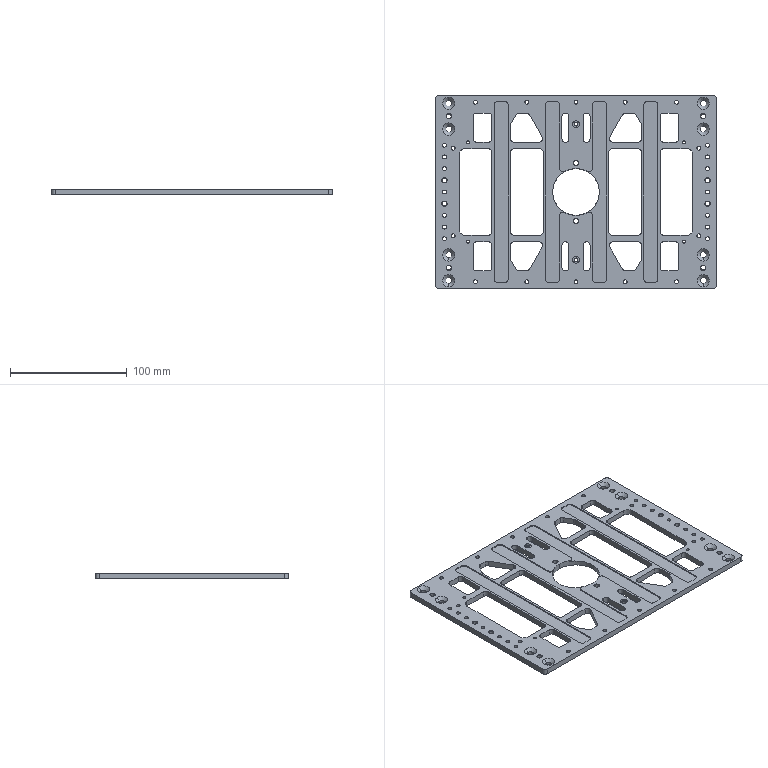NC program | NX | posted with a generic post | part box 240 x 165 x 5 mm
Lines 9636 to 10654 of 12487:
(PLANAR_MILL_COPY_COPY_COPY , TOOL : D6A45)
N19186 T01 M6
N19188 G54
N19190 G17 G0 G90 X-55.05 Y0.866 S9500 M3
N19192 G43 Z30. H1
N19194 Z0.95
N19196 G94 G1 Z-0.55 F1250.
N19198 G3 X-55.55 Y0. R1.
N19200 G1 Y-34.
N19202 G3 X-53. Y-36.55 R2.55
N19204 G1 X-31.
N19206 G3 X-28.45 Y-34. R2.55
N19208 G1 Y34.
N19210 G3 X-31. Y36.55 R2.55
N19212 G1 X-53.
N19214 G3 X-55.55 Y34. R2.55
N19216 G1 Y0.
N19218 G3 X-55.05 Y-0.866 R1.
N19220 G1 Z0.95
N19222 G0 Z30.
N19224 X-69.05 Y0.866
N19226 Z0.95
N19228 G1 Z-0.55
N19230 G3 X-69.55 Y0. R1.
N19232 G1 Y-74.5
N19234 G3 X-67. Y-77.05 R2.55
N19236 G1 X-61.
N19238 G3 X-58.45 Y-74.5 R2.55
N19240 G1 Y74.5
N19242 G3 X-61. Y77.05 R2.55
N19244 G1 X-67.
N19246 G3 X-69.55 Y74.5 R2.55
N19248 G1 Y0.
N19250 G3 X-69.05 Y-0.866 R1.
N19252 G1 Z0.95
N19254 G0 Z30.
N19256 X-99.05 Y0.866
N19258 Z0.95
N19260 G1 Z-0.55
N19262 G3 X-99.55 Y0. R1.
N19264 G1 Y-32.
N19266 G3 X-95. Y-36.55 R4.55
N19268 G1 X-75.
N19270 G3 X-72.45 Y-34. R2.55
N19272 G1 Y34.
N19274 G3 X-75. Y36.55 R2.55
N19276 G1 X-95.
N19278 G3 X-99.55 Y32. R4.55
N19280 G1 Y0.
N19282 G3 X-99.05 Y-0.866 R1.
N19284 G1 Z0.95
N19286 G0 Z30.
N19288 X-93.052 Y42.933
N19290 Z0.95
N19292 G1 Z-0.55
N19294 G3 X-93.302 Y42.5 R0.5
N19296 X-92.502 Y41.7 R0.8
N19298 X-93.302 Y42.5 R-0.8
N19300 X-93.052 Y42.067 R0.5
N19302 G1 Z0.95
N19304 G0 Z30.
N19306 X-87.05 Y55.866
N19308 Z0.95
N19310 G1 Z-0.55
N19312 G3 X-87.55 Y55. R1.
N19314 G1 Y45.5
N19316 G3 X-85. Y42.95 R2.55
N19318 G1 X-75.
N19320 G3 X-72.45 Y45.5 R2.55
N19322 G1 Y64.5
N19324 G3 X-75. Y67.05 R2.55
N19326 G1 X-85.
N19328 G3 X-87.55 Y64.5 R2.55
N19330 G1 Y55.
N19332 G3 X-87.05 Y54.134 R1.
N19334 G1 Z0.95
N19336 G0 Z30.
N19338 X-85.134 Y77.5
N19340 Z0.95
N19342 G1 Z-0.55
N19344 G3 X-86. Y78. R1.
N19346 X-87.2 Y76.8 R1.2
N19348 X-86. Y78. R-1.2
N19350 X-86.866 Y77.5 R1.
N19352 G1 Z0.95
N19354 G0 Z30.
N19356 X-107.884 Y77.45
N19358 Z0.95
N19360 G1 Z-0.55
N19362 G3 X-108.75 Y77.95 R1.
N19364 X-110.95 Y75.75 R2.2
N19366 X-108.75 Y77.95 R-2.2
N19368 X-109.616 Y77.45 R1.
N19370 G1 Z0.95
N19372 G0 Z30.
N19374 X-109.8 Y65.616
N19376 Z0.95
N19378 G1 Z-0.55
N19380 G3 X-110.3 Y64.75 R1.
N19382 X-108.75 Y63.2 R1.55
N19384 X-110.3 Y64.75 R-1.55
N19386 X-109.8 Y63.884 R1.
N19388 G1 Z0.95
N19390 G0 Z30.
N19392 X-110.45 Y54.616
N19394 Z0.95
N19396 G1 Z-0.55
N19398 G3 X-110.95 Y53.75 R1.
N19400 X-108.75 Y51.55 R2.2
N19402 X-110.95 Y53.75 R-2.2
N19404 X-110.45 Y52.884 R1.
N19406 G1 Z0.95
N19408 G0 Z30.
N19410 X-113.2 Y40.866
N19412 Z0.95
N19414 G1 Z-0.55
N19416 G3 X-113.7 Y40. R1.
N19418 X-112.5 Y38.8 R1.2
N19420 X-113.7 Y40. R-1.2
N19422 X-113.2 Y39.134 R1.
N19424 G1 Z0.95
N19426 G0 Z30.
N19428 X-105.7 Y38.366
N19430 Z0.95
N19432 G1 Z-0.55
N19434 G3 X-106.2 Y37.5 R1.
N19436 X-105. Y36.3 R1.2
N19438 X-106.2 Y37.5 R-1.2
N19440 X-105.7 Y36.634 R1.
N19442 G1 Z0.95
N19444 G0 Z30.
N19446 X-113.2 Y30.866
N19448 Z0.95
N19450 G1 Z-0.55
N19452 G3 X-113.7 Y30. R1.
N19454 X-112.5 Y28.8 R1.2
N19456 X-113.7 Y30. R-1.2
N19458 X-113.2 Y29.134 R1.
N19460 G1 Z0.95
N19462 G0 Z30.
N19464 Y20.866
N19466 Z0.95
N19468 G1 Z-0.55
N19470 G3 X-113.7 Y20. R1.
N19472 X-112.5 Y18.8 R1.2
N19474 X-113.7 Y20. R-1.2
N19476 X-113.2 Y19.134 R1.
N19478 G1 Z0.95
N19480 G0 Z30.
N19482 X-113.55 Y10.866
N19484 Z0.95
N19486 G1 Z-0.55
N19488 G3 X-114.05 Y10. R1.
N19490 X-112.5 Y8.45 R1.55
N19492 X-114.05 Y10. R-1.55
N19494 X-113.55 Y9.134 R1.
N19496 G1 Z0.95
N19498 G0 Z30.
N19500 X-113.2 Y0.866
N19502 Z0.95
N19504 G1 Z-0.55
N19506 G3 X-113.7 Y0. R1.
N19508 X-112.5 Y-1.2 R1.2
N19510 X-113.7 Y0. R-1.2
N19512 X-113.2 Y-0.866 R1.
N19514 G1 Z0.95
N19516 G0 Z30.
N19518 X-113.55 Y-9.134
N19520 Z0.95
N19522 G1 Z-0.55
N19524 G3 X-114.05 Y-10. R1.
N19526 X-112.5 Y-11.55 R1.55
N19528 X-114.05 Y-10. R-1.55
N19530 X-113.55 Y-10.866 R1.
N19532 G1 Z0.95
N19534 G0 Z30.
N19536 X-113.2 Y-19.134
N19538 Z0.95
N19540 G1 Z-0.55
N19542 G3 X-113.7 Y-20. R1.
N19544 X-112.5 Y-21.2 R1.2
N19546 X-113.7 Y-20. R-1.2
N19548 X-113.2 Y-20.866 R1.
N19550 G1 Z0.95
N19552 G0 Z30.
N19554 Y-29.134
N19556 Z0.95
N19558 G1 Z-0.55
N19560 G3 X-113.7 Y-30. R1.
N19562 X-112.5 Y-31.2 R1.2
N19564 X-113.7 Y-30. R-1.2
N19566 X-113.2 Y-30.866 R1.
N19568 G1 Z0.95
N19570 G0 Z30.
N19572 Y-39.134
N19574 Z0.95
N19576 G1 Z-0.55
N19578 G3 X-113.7 Y-40. R1.
N19580 X-112.5 Y-41.2 R1.2
N19582 X-113.7 Y-40. R-1.2
N19584 X-113.2 Y-40.866 R1.
N19586 G1 Z0.95
N19588 G0 Z30.
N19590 X-105.7 Y-36.634
N19592 Z0.95
N19594 G1 Z-0.55
N19596 G3 X-106.2 Y-37.5 R1.
N19598 X-105. Y-38.7 R1.2
N19600 X-106.2 Y-37.5 R-1.2
N19602 X-105.7 Y-38.366 R1.
N19604 G1 Z0.95
N19606 G0 Z30.
N19608 X-93.052 Y-42.069
N19610 Z0.95
N19612 G1 Z-0.55
N19614 G3 X-93.302 Y-42.502 R0.5
N19616 X-92.502 Y-43.302 R0.8
N19618 X-93.302 Y-42.502 R-0.8
N19620 X-93.052 Y-42.935 R0.5
N19622 G1 Z0.95
N19624 G0 Z30.
N19626 X-110.45 Y-52.884
N19628 Z0.95
N19630 G1 Z-0.55
N19632 G3 X-110.95 Y-53.75 R1.
N19634 X-108.75 Y-55.95 R2.2
N19636 X-110.95 Y-53.75 R-2.2
N19638 X-110.45 Y-54.616 R1.
N19640 G1 Z0.95
N19642 G0 Z30.
N19644 X-109.8 Y-63.884
N19646 Z0.95
N19648 G1 Z-0.55
N19650 G3 X-110.3 Y-64.75 R1.
N19652 X-108.75 Y-66.3 R1.55
N19654 X-110.3 Y-64.75 R-1.55
N19656 X-109.8 Y-65.616 R1.
N19658 G1 Z0.95
N19660 G0 Z30.
N19662 X-109.616 Y-77.45
N19664 Z0.95
N19666 G1 Z-0.55
N19668 G3 X-108.75 Y-77.95 R1.
N19670 X-106.55 Y-75.75 R2.2
N19672 X-108.75 Y-77.95 R-2.2
N19674 X-107.884 Y-77.45 R1.
N19676 G1 Z0.95
N19678 G0 Z30.
N19680 X-86.866 Y-77.5
N19682 Z0.95
N19684 G1 Z-0.55
N19686 G3 X-86. Y-78. R1.
N19688 X-84.8 Y-76.8 R1.2
N19690 X-86. Y-78. R-1.2
N19692 X-85.134 Y-77.5 R1.
N19694 G1 Z0.95
N19696 G0 Z30.
N19698 X-87.05 Y-54.134
N19700 Z0.95
N19702 G1 Z-0.55
N19704 G3 X-87.55 Y-55. R1.
N19706 G1 Y-64.5
N19708 G3 X-85. Y-67.05 R2.55
N19710 G1 X-75.
N19712 G3 X-72.45 Y-64.5 R2.55
N19714 G1 Y-45.5
N19716 G3 X-75. Y-42.95 R2.55
N19718 G1 X-85.
N19720 G3 X-87.55 Y-45.5 R2.55
N19722 G1 Y-55.
N19724 G3 X-87.05 Y-55.866 R1.
N19726 G1 Z0.95
N19728 G0 Z30.
N19730 X-35.663 Y-56.775
N19732 Z0.95
N19734 G1 Z-0.55
N19736 G3 X-34.797 Y-56.275 R1.
N19738 G1 X-29.312 Y-46.775
N19740 G3 X-31.521 Y-42.95 R2.55
N19742 G1 X-53.
N19744 G3 X-55.55 Y-45.5 R2.55
N19746 G1 Y-56.722
N19748 G3 X-55.208 Y-57.997 R2.55
N19750 G1 X-50.718 Y-65.775
N19752 G3 X-48.51 Y-67.05 R2.55
N19754 G1 X-42.49
N19756 G3 X-40.282 Y-65.775 R2.55
N19758 G1 X-34.797 Y-56.275
N19760 G3 X-34.797 Y-55.275 R1.
N19762 G1 Z0.95
N19764 G0 Z30.
N19766 X-42.866 Y-77.5
N19768 Z0.95
N19770 G1 Z-0.55
N19772 G3 X-42. Y-78. R1.
N19774 X-40.8 Y-76.8 R1.2
N19776 X-42. Y-78. R-1.2
N19778 X-41.134 Y-77.5 R1.
N19780 G1 Z0.95
N19782 G0 Z30.
N19784 X-0.866
N19786 Z0.95
N19788 G1 Z-0.55
N19790 G3 X0. Y-78. R1.
N19792 X1.2 Y-76.8 R1.2
N19794 X0. Y-78. R-1.2
N19796 X0.866 Y-77.5 R1.
N19798 G1 Z0.95
N19800 G0 Z30.
N19802 X-6.95 Y-55.866
N19804 Z0.95
N19806 G1 Z-0.55
N19808 G3 X-6.45 Y-55. R1.
N19810 G1 Y-45.5
N19812 G3 X-9. Y-42.95 R2.55
N19814 X-11.55 Y-45.5 R2.55
N19816 G1 Y-64.5
N19818 G3 X-9. Y-67.05 R2.55
N19820 X-6.45 Y-64.5 R2.55
N19822 G1 Y-55.
N19824 G3 X-6.95 Y-54.134 R1.
N19826 G1 Z0.95
N19828 G0 Z30.
N19830 X-0.866 Y-60.05
N19832 Z0.95
N19834 G1 Z-0.55
N19836 G3 X0. Y-60.55 R1.
N19838 X2.55 Y-58. R2.55
N19840 X0. Y-60.55 R-2.55
N19842 X0.866 Y-60.05 R1.
N19844 G1 Z0.95
N19846 G0 Z30.
N19848 X6.95 Y-54.134
N19850 Z0.95
N19852 G1 Z-0.55
N19854 G3 X6.45 Y-55. R1.
N19856 G1 Y-64.5
N19858 G3 X9. Y-67.05 R2.55
N19860 X11.55 Y-64.5 R2.55
N19862 G1 Y-45.5
N19864 G3 X9. Y-42.95 R2.55
N19866 X6.45 Y-45.5 R2.55
N19868 G1 Y-55.
N19870 G3 X6.95 Y-55.866 R1.
N19872 G1 Z0.95
N19874 G0 Z30.
N19876 X41.134 Y-77.5
N19878 Z0.95
N19880 G1 Z-0.55
N19882 G3 X42. Y-78. R1.
N19884 X43.2 Y-76.8 R1.2
N19886 X42. Y-78. R-1.2
N19888 X42.866 Y-77.5 R1.
N19890 G1 Z0.95
N19892 G0 Z30.
N19894 X34.797 Y-55.275
N19896 Z0.95
N19898 G1 Z-0.55
N19900 G3 X34.797 Y-56.275 R1.
N19902 G1 X40.282 Y-65.775
N19904 G3 X42.49 Y-67.05 R2.55
N19906 G1 X48.51
N19908 G3 X50.718 Y-65.775 R2.55
N19910 G1 X55.208 Y-57.997
N19912 G3 X55.55 Y-56.722 R2.55
N19914 G1 Y-45.5
N19916 G3 X53. Y-42.95 R2.55
N19918 G1 X31.521
N19920 G3 X29.312 Y-46.775 R2.55
N19922 G1 X34.797 Y-56.275
N19924 G3 X35.663 Y-56.775 R1.
N19926 G1 Z0.95
N19928 G0 Z30.
N19930 X72.95 Y-54.134
N19932 Z0.95
N19934 G1 Z-0.55
N19936 G3 X72.45 Y-55. R1.
N19938 G1 Y-64.5
N19940 G3 X75. Y-67.05 R2.55
N19942 G1 X85.
N19944 G3 X87.55 Y-64.5 R2.55
N19946 G1 Y-45.5
N19948 G3 X85. Y-42.95 R2.55
N19950 G1 X75.
N19952 G3 X72.45 Y-45.5 R2.55
N19954 G1 Y-55.
N19956 G3 X72.95 Y-55.866 R1.
N19958 G1 Z0.95
N19960 G0 Z30.
N19962 X85.134 Y-77.5
N19964 Z0.95
N19966 G1 Z-0.55
N19968 G3 X86. Y-78. R1.
N19970 X87.2 Y-76.8 R1.2
N19972 X86. Y-78. R-1.2
N19974 X86.866 Y-77.5 R1.
N19976 G1 Z0.95
N19978 G0 Z30.
N19980 X107.884 Y-77.45
N19982 Z0.95
N19984 G1 Z-0.55
N19986 G3 X108.75 Y-77.95 R1.
N19988 X110.95 Y-75.75 R2.2
N19990 X108.75 Y-77.95 R-2.2
N19992 X109.616 Y-77.45 R1.
N19994 G1 Z0.95
N19996 G0 Z30.
N19998 X109.8 Y-65.616
N20000 Z0.95
N20002 G1 Z-0.55
N20004 G3 X110.3 Y-64.75 R1.
N20006 X108.75 Y-63.2 R1.55
N20008 X110.3 Y-64.75 R-1.55
N20010 X109.8 Y-63.884 R1.
N20012 G1 Z0.95
N20014 G0 Z30.
N20016 X110.45 Y-54.616
N20018 Z0.95
N20020 G1 Z-0.55
N20022 G3 X110.95 Y-53.75 R1.
N20024 X108.75 Y-51.55 R2.2
N20026 X110.95 Y-53.75 R-2.2
N20028 X110.45 Y-52.884 R1.
N20030 G1 Z0.95
N20032 G0 Z30.
N20034 X93.05 Y-42.935
N20036 Z0.95
N20038 G1 Z-0.55
N20040 G3 X93.3 Y-42.502 R0.5
N20042 X92.5 Y-41.702 R0.8
N20044 X93.3 Y-42.502 R-0.8
N20046 X93.05 Y-42.069 R0.5
N20048 G1 Z0.95
N20050 G0 Z30.
N20052 X105.7 Y-38.366
N20054 Z0.95
N20056 G1 Z-0.55
N20058 G3 X106.2 Y-37.5 R1.
N20060 X105. Y-36.3 R1.2
N20062 X106.2 Y-37.5 R-1.2
N20064 X105.7 Y-36.634 R1.
N20066 G1 Z0.95
N20068 G0 Z30.
N20070 X113.2 Y-40.866
N20072 Z0.95
N20074 G1 Z-0.55
N20076 G3 X113.7 Y-40. R1.
N20078 X112.5 Y-38.8 R1.2
N20080 X113.7 Y-40. R-1.2
N20082 X113.2 Y-39.134 R1.
N20084 G1 Z0.95
N20086 G0 Z30.
N20088 Y-30.866
N20090 Z0.95
N20092 G1 Z-0.55
N20094 G3 X113.7 Y-30. R1.
N20096 X112.5 Y-28.8 R1.2
N20098 X113.7 Y-30. R-1.2
N20100 X113.2 Y-29.134 R1.
N20102 G1 Z0.95
N20104 G0 Z30.
N20106 Y-20.866
N20108 Z0.95
N20110 G1 Z-0.55
N20112 G3 X113.7 Y-20. R1.
N20114 X112.5 Y-18.8 R1.2
N20116 X113.7 Y-20. R-1.2
N20118 X113.2 Y-19.134 R1.
N20120 G1 Z0.95
N20122 G0 Z30.
N20124 X113.55 Y-10.866
N20126 Z0.95
N20128 G1 Z-0.55
N20130 G3 X114.05 Y-10. R1.
N20132 X112.5 Y-8.45 R1.55
N20134 X114.05 Y-10. R-1.55
N20136 X113.55 Y-9.134 R1.
N20138 G1 Z0.95
N20140 G0 Z30.
N20142 X113.2 Y-0.866
N20144 Z0.95
N20146 G1 Z-0.55
N20148 G3 X113.7 Y0. R1.
N20150 X112.5 Y1.2 R1.2
N20152 X113.7 Y0. R-1.2
N20154 X113.2 Y0.866 R1.
N20156 G1 Z0.95
N20158 G0 Z30.
N20160 X113.55 Y9.134
N20162 Z0.95
N20164 G1 Z-0.55
N20166 G3 X114.05 Y10. R1.
N20168 X112.5 Y11.55 R1.55
N20170 X114.05 Y10. R-1.55
N20172 X113.55 Y10.866 R1.
N20174 G1 Z0.95
N20176 G0 Z30.
N20178 X113.2 Y19.134
N20180 Z0.95
N20182 G1 Z-0.55
N20184 G3 X113.7 Y20. R1.
N20186 X112.5 Y21.2 R1.2
N20188 X113.7 Y20. R-1.2
N20190 X113.2 Y20.866 R1.
N20192 G1 Z0.95
N20194 G0 Z30.
N20196 Y29.134
N20198 Z0.95
N20200 G1 Z-0.55
N20202 G3 X113.7 Y30. R1.
N20204 X112.5 Y31.2 R1.2
N20206 X113.7 Y30. R-1.2
N20208 X113.2 Y30.866 R1.
N20210 G1 Z0.95
N20212 G0 Z30.
N20214 Y39.134
N20216 Z0.95
N20218 G1 Z-0.55
N20220 G3 X113.7 Y40. R1.
N20222 X112.5 Y41.2 R1.2
N20224 X113.7 Y40. R-1.2
N20226 X113.2 Y40.866 R1.
N20228 G1 Z0.95
N20230 G0 Z30.
N20232 X105.7 Y36.634
N20234 Z0.95
N20236 G1 Z-0.55
N20238 G3 X106.2 Y37.5 R1.
N20240 X105. Y38.7 R1.2
N20242 X106.2 Y37.5 R-1.2
N20244 X105.7 Y38.366 R1.
N20246 G1 Z0.95
N20248 G0 Z30.
N20250 X93.05 Y42.067
N20252 Z0.95
N20254 G1 Z-0.55
N20256 G3 X93.3 Y42.5 R0.5
N20258 X92.5 Y43.3 R0.8
N20260 X93.3 Y42.5 R-0.8
N20262 X93.05 Y42.933 R0.5
N20264 G1 Z0.95
N20266 G0 Z30.
N20268 X110.45 Y52.884
N20270 Z0.95
N20272 G1 Z-0.55
N20274 G3 X110.95 Y53.75 R1.
N20276 X108.75 Y55.95 R2.2
N20278 X110.95 Y53.75 R-2.2
N20280 X110.45 Y54.616 R1.
N20282 G1 Z0.95
N20284 G0 Z30.
N20286 X109.8 Y63.884
N20288 Z0.95
N20290 G1 Z-0.55
N20292 G3 X110.3 Y64.75 R1.
N20294 X108.75 Y66.3 R1.55
N20296 X110.3 Y64.75 R-1.55
N20298 X109.8 Y65.616 R1.
N20300 G1 Z0.95
N20302 G0 Z30.
N20304 X109.616 Y77.45
N20306 Z0.95
N20308 G1 Z-0.55
N20310 G3 X108.75 Y77.95 R1.
N20312 X106.55 Y75.75 R2.2
N20314 X108.75 Y77.95 R-2.2
N20316 X107.884 Y77.45 R1.
N20318 G1 Z0.95
N20320 G0 Z30.
N20322 X86.866 Y77.5
N20324 Z0.95
N20326 G1 Z-0.55
N20328 G3 X86. Y78. R1.
N20330 X84.8 Y76.8 R1.2
N20332 X86. Y78. R-1.2
N20334 X85.134 Y77.5 R1.
N20336 G1 Z0.95
N20338 G0 Z30.
N20340 X87.05 Y54.134
N20342 Z0.95
N20344 G1 Z-0.55
N20346 G3 X87.55 Y55. R1.
N20348 G1 Y64.5
N20350 G3 X85. Y67.05 R2.55
N20352 G1 X75.
N20354 G3 X72.45 Y64.5 R2.55
N20356 G1 Y45.5
N20358 G3 X75. Y42.95 R2.55
N20360 G1 X85.
N20362 G3 X87.55 Y45.5 R2.55
N20364 G1 Y55.
N20366 G3 X87.05 Y55.866 R1.
N20368 G1 Z0.95
N20370 G0 Z30.
N20372 X35.663 Y56.775
N20374 Z0.95
N20376 G1 Z-0.55
N20378 G3 X34.797 Y56.275 R1.
N20380 G1 X29.312 Y46.775
N20382 G3 X31.521 Y42.95 R2.55
N20384 G1 X53.
N20386 G3 X55.55 Y45.5 R2.55
N20388 G1 Y56.722
N20390 G3 X55.208 Y57.997 R2.55
N20392 G1 X50.718 Y65.775
N20394 G3 X48.51 Y67.05 R2.55
N20396 G1 X42.49
N20398 G3 X40.282 Y65.775 R2.55
N20400 G1 X34.797 Y56.275
N20402 G3 X34.797 Y55.275 R1.
N20404 G1 Z0.95
N20406 G0 Z30.
N20408 X42.866 Y77.5
N20410 Z0.95
N20412 G1 Z-0.55
N20414 G3 X42. Y78. R1.
N20416 X40.8 Y76.8 R1.2
N20418 X42. Y78. R-1.2
N20420 X41.134 Y77.5 R1.
N20422 G1 Z0.95
N20424 G0 Z30.
N20426 X0.866
N20428 Z0.95
N20430 G1 Z-0.55
N20432 G3 X0. Y78. R1.
N20434 X-1.2 Y76.8 R1.2
N20436 X0. Y78. R-1.2
N20438 X-0.866 Y77.5 R1.
N20440 G1 Z0.95
N20442 G0 Z30.
N20444 X-41.134
N20446 Z0.95
N20448 G1 Z-0.55
N20450 G3 X-42. Y78. R1.
N20452 X-43.2 Y76.8 R1.2
N20454 X-42. Y78. R-1.2
N20456 X-42.866 Y77.5 R1.
N20458 G1 Z0.95
N20460 G0 Z30.
N20462 X-34.797 Y55.275
N20464 Z0.95
N20466 G1 Z-0.55
N20468 G3 X-34.797 Y56.275 R1.
N20470 G1 X-40.282 Y65.775
N20472 G3 X-42.49 Y67.05 R2.55
N20474 G1 X-48.51
N20476 G3 X-50.718 Y65.775 R2.55
N20478 G1 X-55.208 Y57.997
N20480 G3 X-55.55 Y56.722 R2.55
N20482 G1 Y45.5
N20484 G3 X-53. Y42.95 R2.55
N20486 G1 X-31.521
N20488 G3 X-29.312 Y46.775 R2.55
N20490 G1 X-34.797 Y56.275
N20492 G3 X-35.663 Y56.775 R1.
N20494 G1 Z0.95
N20496 G0 Z30.
N20498 X-11.05 Y55.866
N20500 Z0.95
N20502 G1 Z-0.55
N20504 G3 X-11.55 Y55. R1.
N20506 G1 Y45.5
N20508 G3 X-9. Y42.95 R2.55
N20510 X-6.45 Y45.5 R2.55
N20512 G1 Y64.5
N20514 G3 X-9. Y67.05 R2.55
N20516 X-11.55 Y64.5 R2.55
N20518 G1 Y55.
N20520 G3 X-11.05 Y54.134 R1.
N20522 G1 Z0.95
N20524 G0 Z30.
N20526 X0.866 Y60.05
N20528 Z0.95
N20530 G1 Z-0.55
N20532 G3 X0. Y60.55 R1.
N20534 X-2.55 Y58. R2.55
N20536 X0. Y60.55 R-2.55
N20538 X-0.866 Y60.05 R1.
N20540 G1 Z0.95
N20542 G0 Z30.
N20544 X6.95 Y55.866
N20546 Z0.95
N20548 G1 Z-0.55
N20550 G3 X6.45 Y55. R1.
N20552 G1 Y45.5
N20554 G3 X9. Y42.95 R2.55
N20556 X11.55 Y45.5 R2.55
N20558 G1 Y64.5
N20560 G3 X9. Y67.05 R2.55
N20562 X6.45 Y64.5 R2.55
N20564 G1 Y55.
N20566 G3 X6.95 Y54.134 R1.
N20568 G1 Z0.95
N20570 G0 Z30.
N20572 X0.866 Y26.05
N20574 Z0.95
N20576 G1 Z-0.55
N20578 G3 X0. Y26.55 R1.
N20580 X-1.55 Y25. R1.55
N20582 X0. Y26.55 R-1.55
N20584 X-0.866 Y26.05 R1.
N20586 G1 Z0.95
N20588 G0 Z30.
N20590 X-25.05 Y0.866
N20592 Z0.95
N20594 G1 Z-0.55
N20596 G3 X-25.55 Y0. R1.
N20598 G1 Y-74.5
N20600 G3 X-23. Y-77.05 R2.55
N20602 G1 X-17.
N20604 G3 X-14.45 Y-74.5 R2.55
N20606 G1 Y-20.199
N20608 G2 X-9.35 Y-17.169 R3.45
N20610 G3 X9.35 Y-17.169 R19.55
N20612 G2 X14.45 Y-20.199 R3.45
N20614 G1 Y-74.5
N20616 G3 X17. Y-77.05 R2.55
N20618 G1 X23.
N20620 G3 X25.55 Y-74.5 R2.55
N20622 G1 Y74.5
N20624 G3 X23. Y77.05 R2.55
N20626 G1 X17.
N20628 G3 X14.45 Y74.5 R2.55
N20630 G1 Y20.199
N20632 G2 X9.35 Y17.169 R3.45
N20634 G3 X-9.35 Y17.169 R19.55
N20636 G2 X-14.45 Y20.199 R3.45
N20638 G1 Y74.5
N20640 G3 X-17. Y77.05 R2.55
N20642 G1 X-23.
N20644 G3 X-25.55 Y74.5 R2.55
N20646 G1 Y0.
N20648 G3 X-25.05 Y-0.866 R1.
N20650 G1 Z0.95
N20652 G0 Z30.
N20654 X-0.866 Y83.45
N20656 Z0.95
N20658 G1 Z-0.55
N20660 G3 X0. Y82.95 R1.
N20662 G1 X117.
N20664 G2 X120.45 Y79.5 R3.45
N20666 G1 Y-79.5
N20668 G2 X117. Y-82.95 R3.45
N20670 G1 X-117.
N20672 G2 X-120.45 Y-79.5 R3.45
N20674 G1 Y79.5
N20676 G2 X-117. Y82.95 R3.45
N20678 G1 X0.
N20680 G3 X0.866 Y83.45 R1.
N20682 G1 Z0.95
N20684 G0 Z30.
N20686 X-0.866 Y-26.05
N20688 Z0.95
N20690 G1 Z-0.55
N20692 G3 X0. Y-26.55 R1.
N20694 X1.55 Y-25. R1.55
N20696 X0. Y-26.55 R-1.55
N20698 X0.866 Y-26.05 R1.
N20700 G1 Z0.95
N20702 G0 Z30.
N20704 X55.05 Y-0.866
N20706 Z0.95
N20708 G1 Z-0.55
N20710 G3 X55.55 Y0. R1.
N20712 G1 Y34.
N20714 G3 X53. Y36.55 R2.55
N20716 G1 X31.
N20718 G3 X28.45 Y34. R2.55
N20720 G1 Y-34.
N20722 G3 X31. Y-36.55 R2.55
N20724 G1 X53.
N20726 G3 X55.55 Y-34. R2.55
N20728 G1 Y0.
N20730 G3 X55.05 Y0.866 R1.
N20732 G1 Z0.95
N20734 G0 Z30.
N20736 X69.05 Y-0.866
N20738 Z0.95
N20740 G1 Z-0.55
N20742 G3 X69.55 Y0. R1.
N20744 G1 Y74.5
N20746 G3 X67. Y77.05 R2.55
N20748 G1 X61.
N20750 G3 X58.45 Y74.5 R2.55
N20752 G1 Y-74.5
N20754 G3 X61. Y-77.05 R2.55
N20756 G1 X67.
N20758 G3 X69.55 Y-74.5 R2.55
N20760 G1 Y0.
N20762 G3 X69.05 Y0.866 R1.
N20764 G1 Z0.95
N20766 G0 Z30.
N20768 X99.05 Y-0.866
N20770 Z0.95
N20772 G1 Z-0.55
N20774 G3 X99.55 Y0. R1.
N20776 G1 Y32.
N20778 G3 X95. Y36.55 R4.55
N20780 G1 X75.
N20782 G3 X72.45 Y34. R2.55
N20784 G1 Y-34.
N20786 G3 X75. Y-36.55 R2.55
N20788 G1 X95.
N20790 G3 X99.55 Y-32. R4.55
N20792 G1 Y0.
N20794 G3 X99.05 Y0.866 R1.
N20796 G1 Z0.95
N20798 G0 Z30.
(ZLEVEL_PROFILE_COPY_COPY_1_COPY_1 , TOOL : D6A45)
N20800 X-111.347 Y50.645
N20802 Z1.5
N20804 G1 X-110.82 Y50.216 Z1.464 F1000.
N20806 X-109.656 Y49.756 Z1.399
N20808 X-108.408 Y49.669 Z1.333
N20810 X-107.192 Y49.963 Z1.268
N20812 X-106.329 Y50.447 Z1.216
N20814 X-105.44 Y51.338 Z1.15
N20816 X-104.864 Y52.458 Z1.084
N20818 X-104.655 Y53.7 Z1.018
N20820 X-104.833 Y54.947 Z0.952
N20822 X-105.382 Y56.08 Z0.886
N20824 X-106.249 Y56.993 Z0.82
N20826 X-107.1 Y57.498 Z0.768
N20828 X-108.317 Y57.823 Z0.702
N20830 X-109.574 Y57.762 Z0.636
N20832 X-110.754 Y57.322 Z0.57
N20834 X-111.745 Y56.544 Z0.504
N20836 X-112.452 Y55.502 Z0.438
N20838 X-112.809 Y54.295 Z0.372
N20840 X-112.816 Y53.75 Z0.344
N20842 Y53.255 Z0.318
N20844 X-112.477 Y52.051 Z0.252
N20846 X-111.79 Y51.005 Z0.186
N20848 X-110.82 Y50.216 Z0.121
N20850 X-109.656 Y49.756 Z0.055
N20852 X-108.408 Y49.669 Z-0.01
N20854 X-107.192 Y49.963 Z-0.076
N20856 X-106.329 Y50.447 Z-0.128
N20858 X-105.44 Y51.338 Z-0.194
N20860 X-104.864 Y52.458 Z-0.26
N20862 X-104.655 Y53.7 Z-0.326
N20864 X-104.833 Y54.947 Z-0.392
N20866 X-105.382 Y56.08 Z-0.458
N20868 X-106.249 Y56.993 Z-0.524
N20870 X-107.1 Y57.498 Z-0.575
N20872 X-108.317 Y57.823 Z-0.641
N20874 X-109.574 Y57.762 Z-0.707
N20876 X-110.754 Y57.322 Z-0.773
N20878 X-111.745 Y56.544 Z-0.839
N20880 X-112.452 Y55.502 Z-0.905
N20882 X-112.809 Y54.295 Z-0.971
N20884 X-112.816 Y53.75 Z-1.
N20886 G3 X-108.75 Y49.685 R4.066 F1200.
N20888 X-112.816 Y53.75 R-4.066
N20890 G1 X-112.798 Y53.378 Z-1.016
N20892 X-112.762 Y53.197 Z-1.025
N20894 X-112.668 Y52.827 Z-1.042
N20896 X-112.559 Y52.458 Z-1.059
N20898 X-112.421 Y52.182 Z-1.072
N20900 X-112.315 Y51.972 Z-1.083
N20902 X-112.131 Y51.657 Z-1.099
N20904 X-111.941 Y51.418 Z-1.113
N20906 X-111.782 Y51.227 Z-1.124
N20908 X-111.529 Y50.97 Z-1.14
N20910 X-111.296 Y50.778 Z-1.153
N20912 X-111.1 Y50.629 Z-1.164
N20914 X-110.632 Y50.359 Z-1.189
N20916 X-110.308 Y50.206 Z-1.205
N20918 X-109.889 Y50.08 Z-1.224
N20920 X-109.445 Y49.988 Z-1.244
N20922 X-108.762 Y49.948 Z-1.275
N20924 X-108.566 Y49.968 Z-1.284
N20926 X-107.979 Y50.053 Z-1.31
N20928 X-107.714 Y50.148 Z-1.323
N20930 X-107.332 Y50.292 Z-1.341
N20932 X-107.149 Y50.381 Z-1.35
N20934 X-106.935 Y50.514 Z-1.362
N20936 X-106.612 Y50.724 Z-1.379
N20938 X-106.469 Y50.85 Z-1.387
N20940 X-106.263 Y51.048 Z-1.4
N20942 X-106.012 Y51.304 Z-1.416
N20944 X-105.856 Y51.54 Z-1.429
N20946 X-105.738 Y51.716 Z-1.438
N20948 X-105.568 Y52.006 Z-1.453
N20950 X-105.466 Y52.266 Z-1.466
N20952 X-105.385 Y52.478 Z-1.476
N20954 X-105.269 Y52.945 Z-1.498
N20956 X-105.219 Y53.294 Z-1.514
N20958 X-105.215 Y53.784 Z-1.536
N20960 X-105.238 Y54.117 Z-1.551
N20962 X-105.33 Y54.505 Z-1.569
N20964 X-105.457 Y54.904 Z-1.587
N20966 X-105.606 Y55.215 Z-1.603
N20968 X-105.742 Y55.478 Z-1.616
N20970 X-105.842 Y55.612 Z-1.624
N20972 X-106.205 Y56.065 Z-1.65
N20974 X-106.374 Y56.208 Z-1.66
N20976 X-106.824 Y56.55 Z-1.685
N20978 X-107.023 Y56.66 Z-1.695
N20980 X-107.325 Y56.811 Z-1.71
N20982 X-107.484 Y56.867 Z-1.718
N20984 X-107.751 Y56.947 Z-1.73
N20986 X-108.217 Y57.035 Z-1.752
N20988 X-108.517 Y57.06 Z-1.765
N20990 X-108.963 Y57.035 Z-1.785
N20992 X-109.282 Y56.996 Z-1.8
N20994 X-109.679 Y56.873 Z-1.818
N20996 X-110.006 Y56.762 Z-1.834
N20998 X-110.652 Y56.371 Z-1.867
N21000 X-111.177 Y55.837 Z-1.901
N21002 X-111.502 Y55.349 Z-1.927
N21004 X-111.526 Y55.274 Z-1.93
N21006 X-111.561 Y55.205 Z-1.934
N21008 X-111.701 Y54.802 Z-1.953
N21010 X-111.789 Y54.51 Z-1.966
N21012 X-111.839 Y54.013 Z-1.988
N21014 X-111.851 Y53.788 Z-1.998
N21016 X-111.838 Y53.769 Z-1.999
N21018 X-111.836 Y53.75 Z-2.
N21020 X-111.808 Y53.431 Z-2.019
N21022 X-111.738 Y53.174 Z-2.035
N21024 X-111.698 Y52.962 Z-2.048
N21026 X-111.367 Y52.244 Z-2.096
N21028 X-110.845 Y51.663 Z-2.143
N21030 X-110.521 Y51.425 Z-2.167
N21032 X-110.214 Y51.228 Z-2.19
N21034 X-109.837 Y51.084 Z-2.214
N21036 X-109.502 Y50.976 Z-2.235
N21038 X-109.132 Y50.94 Z-2.258
N21040 X-108.759 Y50.916 Z-2.281
N21042 X-108.2 Y51.001 Z-2.315
N21044 X-108.035 Y51.049 Z-2.326
N21046 X-107.615 Y51.221 Z-2.353
N21048 X-107.38 Y51.36 Z-2.37
N21050 X-107.152 Y51.521 Z-2.387
N21052 X-106.982 Y51.687 Z-2.402
N21054 X-106.839 Y51.828 Z-2.414
N21056 X-106.66 Y52.045 Z-2.431
N21058 X-106.533 Y52.242 Z-2.445
N21060 X-106.434 Y52.405 Z-2.457
N21062 X-106.329 Y52.655 Z-2.473
N21064 X-106.245 Y52.871 Z-2.488
N21066 X-106.203 Y53.06 Z-2.499
N21068 X-106.141 Y53.432 Z-2.522
N21070 X-106.167 Y53.744 Z-2.541
N21072 X-106.233 Y54.282 Z-2.575
N21074 X-106.27 Y54.408 Z-2.583
N21076 X-106.363 Y54.665 Z-2.599
N21078 X-106.464 Y54.862 Z-2.613
N21080 X-106.555 Y55.01 Z-2.624
N21082 X-106.708 Y55.205 Z-2.639
N21084 X-106.875 Y55.391 Z-2.654
N21086 X-106.922 Y55.456 Z-2.659
N21088 X-106.996 Y55.496 Z-2.664
N21090 X-107.111 Y55.609 Z-2.674
N21092 X-107.235 Y55.712 Z-2.684
N21094 X-107.371 Y55.797 Z-2.694
N21096 X-107.524 Y55.862 Z-2.704
N21098 X-108.005 Y56.073 Z-2.736
N21100 X-108.121 Y56.076 Z-2.743
N21102 X-108.271 Y56.127 Z-2.752
N21104 X-108.427 Y56.136 Z-2.762
N21106 X-108.584 Y56.144 Z-2.772
N21108 X-108.744 Y56.121 Z-2.781
N21110 X-108.9 Y56.129 Z-2.791
N21112 X-109.052 Y56.106 Z-2.8
N21114 X-109.203 Y56.082 Z-2.81
N21116 X-109.349 Y56.009 Z-2.819
N21118 X-109.5 Y55.978 Z-2.828
N21120 X-109.641 Y55.924 Z-2.838
N21122 X-109.776 Y55.854 Z-2.847
N21124 X-109.894 Y55.744 Z-2.856
N21126 X-110.037 Y55.686 Z-2.865
N21128 X-110.151 Y55.592 Z-2.875
N21130 X-110.259 Y55.488 Z-2.884
N21132 X-110.339 Y55.349 Z-2.893
N21134 X-110.42 Y55.318 Z-2.897
N21136 X-110.513 Y55.205 Z-2.907
N21138 X-110.548 Y55.139 Z-2.911
N21140 X-110.632 Y55.019 Z-2.92
N21142 X-110.686 Y54.875 Z-2.929
N21144 X-110.763 Y54.789 Z-2.936
N21146 X-110.803 Y54.685 Z-2.943
N21148 X-110.843 Y54.581 Z-2.949
N21150 X-110.866 Y54.47 Z-2.956
N21152 X-110.888 Y54.402 Z-2.961
N21154 X-110.874 Y54.323 Z-2.965
N21156 X-110.933 Y54.04 Z-2.982
N21158 X-110.942 Y53.75 Z-3.
N21160 G3 X-108.748 Y51.555 R2.195
N21162 X-110.942 Y53.75 R-2.195
N21164 G1 Z-1.5
N21166 G0 Z30.
N21168 X-111.857 Y78.353
N21170 Z1.5
N21172 G1 X-112.448 Y77.51 Z1.446 F1000.
N21174 X-112.821 Y76.196 Z1.374
N21176 X-112.809 Y75.207 Z1.323
N21178 X-112.452 Y73.999 Z1.257
N21180 X-111.745 Y72.957 Z1.191
N21182 X-110.754 Y72.179 Z1.125
N21184 X-109.575 Y71.739 Z1.059
N21186 X-108.317 Y71.678 Z0.993
N21188 X-107.1 Y72.002 Z0.927
N21190 X-106.249 Y72.507 Z0.875
N21192 X-105.382 Y73.42 Z0.809
N21194 X-104.833 Y74.553 Z0.743
N21196 X-104.654 Y75.8 Z0.677
N21198 X-104.863 Y77.042 Z0.611
N21200 X-105.439 Y78.162 Z0.545
N21202 X-106.328 Y79.053 Z0.479
N21204 X-107.191 Y79.538 Z0.427
N21206 X-108.255 Y79.816 Z0.369
N21208 X-109.244 Z0.317
N21210 X-110.554 Y79.427 Z0.246